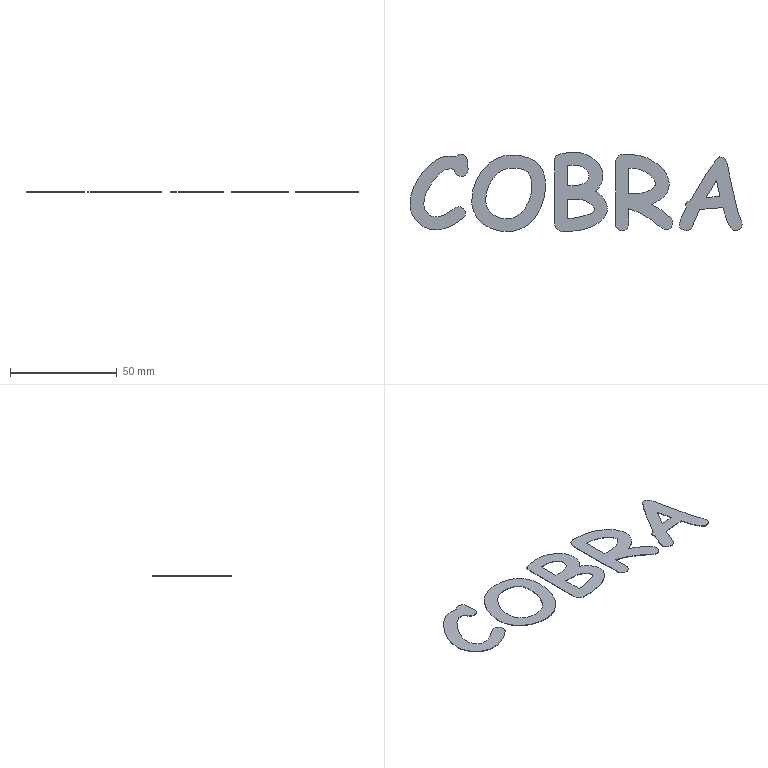Part | STEP file | Cobra sign | 5 solids | 119 faces | box 155.556 x 37.16 x 0.2 mm | volume 521.98 mm3 | spline 103 | plane 16